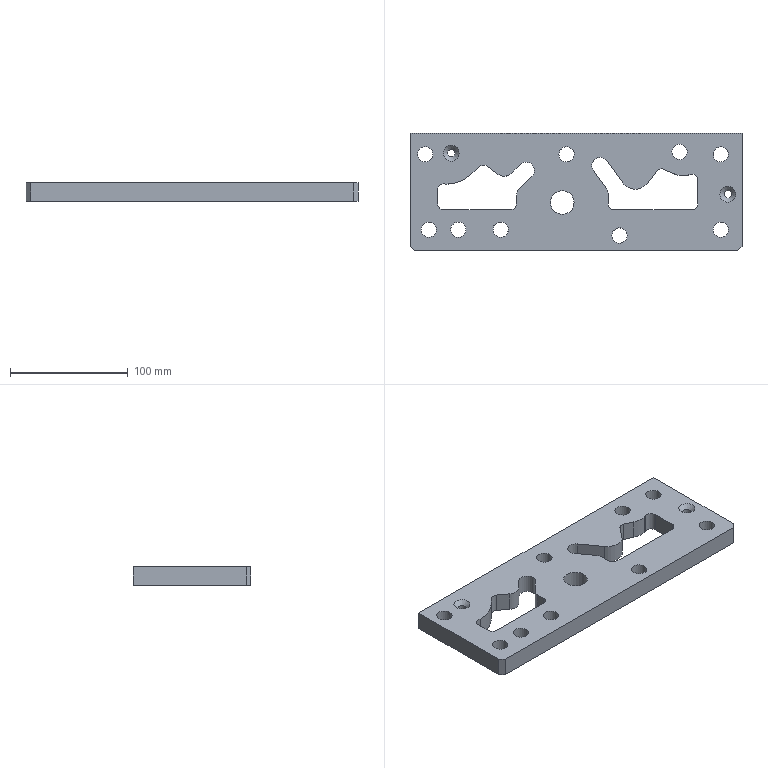Part | STEP file | gslz 2016.10.28-13_id122_x_t | 1 solid | 54 faces | box 282 x 100 x 16 mm | volume 353855 mm3 | cylinder 29 | plane 23 | cone 2 | commonest cylinder face diameters 13 x9 10 x8 14 x4 6.5 x2 18 x1 20 x1